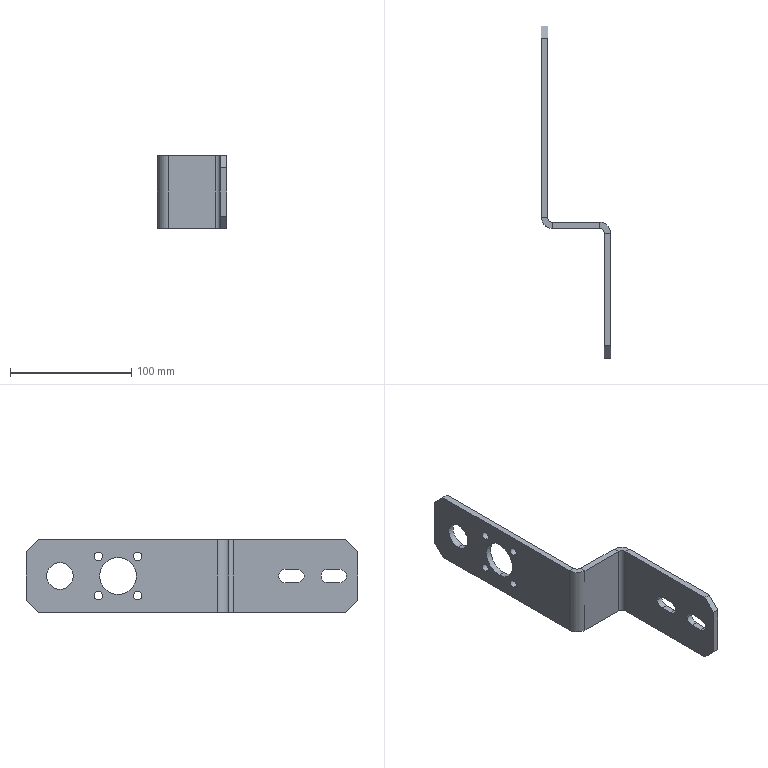Part | STEP file | BCC3 H14_3B | 1 solid | 48 faces | box 57 x 274 x 60 mm | volume 86752 mm3 | plane 26 | cylinder 22 | commonest cylinder face diameters 7 x8 11 x6 8 x2 18 x2 22 x2 30.5 x2